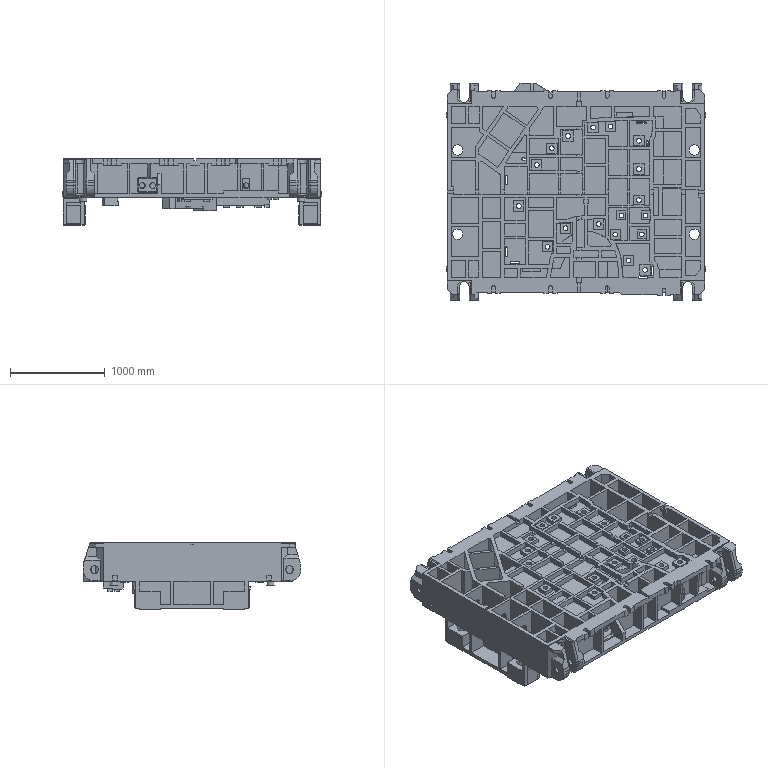Part | NX | features solid 2 | 1 solid | 2266 faces | box 2740 x 2301 x 705 mm | volume 886809609 mm3 | plane 1883 | cylinder 309 | spline 53 | torus 20 | cone 1 | commonest cylinder face diameters 40 x55 83 x48 80 x41 20 x32 100 x21 79 x16